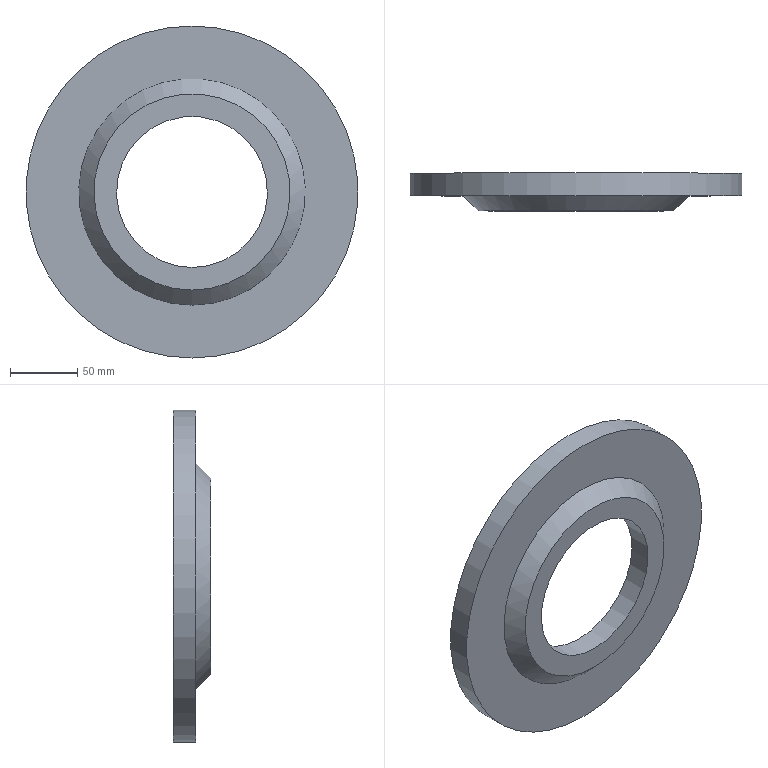Part | NX | features DATUM_CSYS 1, Delete Body 1, LINKED_BODY 1, SCALE 1, SKETCH 1, SWP104 1 | 1 solid | 8 faces | box 247.5 x 28.125 x 247.5 mm | volume 674318 mm3 | plane 4 | cone 2 | cylinder 2 | commonest cylinder face diameters 112.5 x1 247.5 x1
STEP:
#1=CARTESIAN_POINT('',(2029.479,-116.,-439.707));
#2=VERTEX_POINT('',#1);
#3=CARTESIAN_POINT('',(2029.479,-116.,-366.582));
#4=DIRECTION('',(0.,-1.,0.));
#5=DIRECTION('',(0.,0.,-1.));
#6=AXIS2_PLACEMENT_3D('',#3,#4,#5);
#7=CIRCLE('',#6,73.125);
#8=EDGE_CURVE('',#2,#2,#7,.T.);
#9=ORIENTED_EDGE('',*,*,#8,.F.);
#10=EDGE_LOOP('',(#9));
#11=FACE_BOUND('',#10,.T.);
#12=CARTESIAN_POINT('',(2029.479,-104.75,-450.957));
#13=VERTEX_POINT('',#12);
#14=CARTESIAN_POINT('',(2029.479,-104.75,-366.582));
#15=DIRECTION('',(0.,-1.,0.));
#16=DIRECTION('',(0.,0.,-1.));
#17=AXIS2_PLACEMENT_3D('',#14,#15,#16);
#18=CIRCLE('',#17,84.375);
#19=EDGE_CURVE('',#13,#13,#18,.T.);
#20=ORIENTED_EDGE('',*,*,#19,.T.);
#21=EDGE_LOOP('',(#20));
#22=FACE_BOUND('',#21,.T.);
#23=CARTESIAN_POINT('',(2029.479,-104.75,-366.582));
#24=DIRECTION('',(0.,1.,0.));
#25=DIRECTION('',(0.,0.,1.));
#26=AXIS2_PLACEMENT_3D('',#23,#24,#25);
#27=CONICAL_SURFACE('',#26,84.375,0.7854);
#28=ADVANCED_FACE('',(#11,#22),#27,.T.);
#29=CARTESIAN_POINT('',(2029.479,-116.,-422.832));
#30=VERTEX_POINT('',#29);
#31=CARTESIAN_POINT('',(2029.479,-116.,-366.582));
#32=DIRECTION('',(0.,-1.,0.));
#33=DIRECTION('',(0.,0.,-1.));
#34=AXIS2_PLACEMENT_3D('',#31,#32,#33);
#35=CIRCLE('',#34,56.25);
#36=EDGE_CURVE('',#30,#30,#35,.T.);
#37=ORIENTED_EDGE('',*,*,#36,.F.);
#38=EDGE_LOOP('',(#37));
#39=FACE_BOUND('',#38,.T.);
#40=ORIENTED_EDGE('',*,*,#8,.T.);
#41=EDGE_LOOP('',(#40));
#42=FACE_BOUND('',#41,.T.);
#43=CARTESIAN_POINT('',(2029.479,-116.,-293.457));
#44=DIRECTION('',(0.,1.,0.));
#45=DIRECTION('',(0.,0.,1.));
#46=AXIS2_PLACEMENT_3D('',#43,#44,#45);
#47=PLANE('',#46);
#48=ADVANCED_FACE('',(#39,#42),#47,.F.);
#49=CARTESIAN_POINT('',(2029.479,-99.125,-422.832));
#50=VERTEX_POINT('',#49);
#51=CARTESIAN_POINT('',(2029.479,-99.125,-366.582));
#52=DIRECTION('',(0.,-1.,0.));
#53=DIRECTION('',(0.,0.,-1.));
#54=AXIS2_PLACEMENT_3D('',#51,#52,#53);
#55=CIRCLE('',#54,56.25);
#56=EDGE_CURVE('',#50,#50,#55,.T.);
#57=ORIENTED_EDGE('',*,*,#56,.F.);
#58=EDGE_LOOP('',(#57));
#59=FACE_BOUND('',#58,.T.);
#60=ORIENTED_EDGE('',*,*,#36,.T.);
#61=EDGE_LOOP('',(#60));
#62=FACE_BOUND('',#61,.T.);
#63=CARTESIAN_POINT('',(2029.479,-116.,-366.582));
#64=DIRECTION('',(0.,-1.,0.));
#65=DIRECTION('',(0.,0.,-1.));
#66=AXIS2_PLACEMENT_3D('',#63,#64,#65);
#67=CYLINDRICAL_SURFACE('',#66,56.25);
#68=ADVANCED_FACE('',(#59,#62),#67,.F.);
#69=CARTESIAN_POINT('',(2029.479,-99.125,-434.082));
#70=VERTEX_POINT('',#69);
#71=CARTESIAN_POINT('',(2029.479,-99.125,-366.582));
#72=DIRECTION('',(0.,-1.,0.));
#73=DIRECTION('',(0.,0.,-1.));
#74=AXIS2_PLACEMENT_3D('',#71,#72,#73);
#75=CIRCLE('',#74,67.5);
#76=EDGE_CURVE('',#70,#70,#75,.T.);
#77=ORIENTED_EDGE('',*,*,#76,.F.);
#78=EDGE_LOOP('',(#77));
#79=FACE_BOUND('',#78,.T.);
#80=ORIENTED_EDGE('',*,*,#56,.T.);
#81=EDGE_LOOP('',(#80));
#82=FACE_BOUND('',#81,.T.);
#83=CARTESIAN_POINT('',(2029.479,-99.125,-310.332));
#84=DIRECTION('',(0.,-1.,0.));
#85=DIRECTION('',(0.,0.,-1.));
#86=AXIS2_PLACEMENT_3D('',#83,#84,#85);
#87=PLANE('',#86);
#88=ADVANCED_FACE('',(#79,#82),#87,.F.);
#89=CARTESIAN_POINT('',(2029.479,-87.875,-445.332));
#90=VERTEX_POINT('',#89);
#91=CARTESIAN_POINT('',(2029.479,-87.875,-366.582));
#92=DIRECTION('',(0.,-1.,0.));
#93=DIRECTION('',(0.,0.,-1.));
#94=AXIS2_PLACEMENT_3D('',#91,#92,#93);
#95=CIRCLE('',#94,78.75);
#96=EDGE_CURVE('',#90,#90,#95,.T.);
#97=ORIENTED_EDGE('',*,*,#96,.F.);
#98=EDGE_LOOP('',(#97));
#99=FACE_BOUND('',#98,.T.);
#100=ORIENTED_EDGE('',*,*,#76,.T.);
#101=EDGE_LOOP('',(#100));
#102=FACE_BOUND('',#101,.T.);
#103=CARTESIAN_POINT('',(2029.479,-99.125,-366.582));
#104=DIRECTION('',(0.,1.,0.));
#105=DIRECTION('',(0.,0.,1.));
#106=AXIS2_PLACEMENT_3D('',#103,#104,#105);
#107=CONICAL_SURFACE('',#106,67.5,0.7854);
#108=ADVANCED_FACE('',(#99,#102),#107,.F.);
#109=CARTESIAN_POINT('',(2029.479,-87.875,-490.332));
#110=VERTEX_POINT('',#109);
#111=CARTESIAN_POINT('',(2029.479,-87.875,-366.582));
#112=DIRECTION('',(0.,-1.,0.));
#113=DIRECTION('',(0.,0.,-1.));
#114=AXIS2_PLACEMENT_3D('',#111,#112,#113);
#115=CIRCLE('',#114,123.75);
#116=EDGE_CURVE('',#110,#110,#115,.T.);
#117=ORIENTED_EDGE('',*,*,#116,.F.);
#118=EDGE_LOOP('',(#117));
#119=FACE_BOUND('',#118,.T.);
#120=ORIENTED_EDGE('',*,*,#96,.T.);
#121=EDGE_LOOP('',(#120));
#122=FACE_BOUND('',#121,.T.);
#123=CARTESIAN_POINT('',(2029.479,-87.875,-287.832));
#124=DIRECTION('',(0.,-1.,0.));
#125=DIRECTION('',(0.,0.,-1.));
#126=AXIS2_PLACEMENT_3D('',#123,#124,#125);
#127=PLANE('',#126);
#128=ADVANCED_FACE('',(#119,#122),#127,.F.);
#129=CARTESIAN_POINT('',(2029.479,-104.75,-490.332));
#130=VERTEX_POINT('',#129);
#131=CARTESIAN_POINT('',(2029.479,-104.75,-366.582));
#132=DIRECTION('',(0.,-1.,0.));
#133=DIRECTION('',(0.,0.,-1.));
#134=AXIS2_PLACEMENT_3D('',#131,#132,#133);
#135=CIRCLE('',#134,123.75);
#136=EDGE_CURVE('',#130,#130,#135,.T.);
#137=ORIENTED_EDGE('',*,*,#136,.F.);
#138=EDGE_LOOP('',(#137));
#139=FACE_BOUND('',#138,.T.);
#140=ORIENTED_EDGE('',*,*,#116,.T.);
#141=EDGE_LOOP('',(#140));
#142=FACE_BOUND('',#141,.T.);
#143=CARTESIAN_POINT('',(2029.479,-116.,-366.582));
#144=DIRECTION('',(0.,-1.,0.));
#145=DIRECTION('',(0.,0.,-1.));
#146=AXIS2_PLACEMENT_3D('',#143,#144,#145);
#147=CYLINDRICAL_SURFACE('',#146,123.75);
#148=ADVANCED_FACE('',(#139,#142),#147,.T.);
#149=ORIENTED_EDGE('',*,*,#19,.F.);
#150=EDGE_LOOP('',(#149));
#151=FACE_BOUND('',#150,.T.);
#152=ORIENTED_EDGE('',*,*,#136,.T.);
#153=EDGE_LOOP('',(#152));
#154=FACE_BOUND('',#153,.T.);
#155=CARTESIAN_POINT('',(2029.479,-104.75,-242.832));
#156=DIRECTION('',(0.,1.,0.));
#157=DIRECTION('',(0.,0.,1.));
#158=AXIS2_PLACEMENT_3D('',#155,#156,#157);
#159=PLANE('',#158);
#160=ADVANCED_FACE('',(#151,#154),#159,.F.);
#161=CLOSED_SHELL('',(#28,#48,#68,#88,#108,#128,#148,#160));
#162=MANIFOLD_SOLID_BREP('',#161);
#163=(LENGTH_UNIT()NAMED_UNIT(*)SI_UNIT(.MILLI.,.METRE.));
#164=UNCERTAINTY_MEASURE_WITH_UNIT(LENGTH_MEASURE(0.00001),#163,'','');
#165=(NAMED_UNIT(*)PLANE_ANGLE_UNIT()SI_UNIT($,.RADIAN.));
#166=(NAMED_UNIT(*)SI_UNIT($,.STERADIAN.)SOLID_ANGLE_UNIT());
#167=(GEOMETRIC_REPRESENTATION_CONTEXT(3)GLOBAL_UNCERTAINTY_ASSIGNED_CONTEXT((#164))GLOBAL_UNIT_ASSIGNED_CONTEXT((#163,#165,#166))REPRESENTATION_CONTEXT('',''));
#168=ADVANCED_BREP_SHAPE_REPRESENTATION('',(#162),#167);